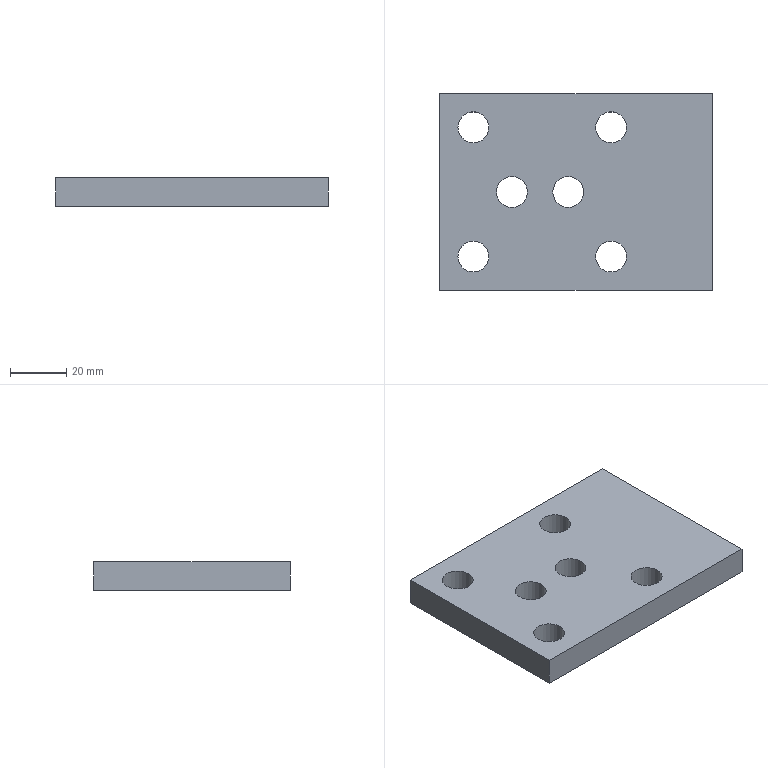Part | NX | features solid 2 | 1 solid | 12 faces | box 97 x 70 x 10 mm | volume 62198 mm3 | plane 6 | cylinder 6 | commonest cylinder face diameters 11 x6
STEP:
#1=CARTESIAN_POINT('',(1618.396,35.,88.));
#2=VERTEX_POINT('',#1);
#3=CARTESIAN_POINT('',(1618.396,35.,78.));
#4=VERTEX_POINT('',#3);
#5=CARTESIAN_POINT('',(1618.396,35.,78.));
#6=DIRECTION('',(0.,0.,1.));
#7=VECTOR('',#6,1000.);
#8=LINE('',#5,#7);
#9=EDGE_CURVE('',#2,#4,#8,.F.);
#10=ORIENTED_EDGE('',*,*,#9,.T.);
#11=CARTESIAN_POINT('',(1521.396,35.,78.));
#12=VERTEX_POINT('',#11);
#13=CARTESIAN_POINT('',(1569.896,35.,78.));
#14=DIRECTION('',(-1.,0.,0.));
#15=VECTOR('',#14,1000.);
#16=LINE('',#13,#15);
#17=EDGE_CURVE('',#12,#4,#16,.F.);
#18=ORIENTED_EDGE('',*,*,#17,.F.);
#19=CARTESIAN_POINT('',(1521.396,35.,88.));
#20=VERTEX_POINT('',#19);
#21=CARTESIAN_POINT('',(1521.396,35.,78.));
#22=DIRECTION('',(0.,0.,1.));
#23=VECTOR('',#22,1000.);
#24=LINE('',#21,#23);
#25=EDGE_CURVE('',#20,#12,#24,.F.);
#26=ORIENTED_EDGE('',*,*,#25,.F.);
#27=CARTESIAN_POINT('',(2186.158,35.,88.));
#28=DIRECTION('',(1.,0.,0.));
#29=VECTOR('',#28,1000.);
#30=LINE('',#27,#29);
#31=EDGE_CURVE('',#20,#2,#30,.T.);
#32=ORIENTED_EDGE('',*,*,#31,.T.);
#33=EDGE_LOOP('',(#10,#18,#26,#32));
#34=FACE_BOUND('',#33,.T.);
#35=CARTESIAN_POINT('',(1569.896,35.,78.));
#36=DIRECTION('',(0.,-1.,0.));
#37=DIRECTION('',(-1.,0.,0.));
#38=AXIS2_PLACEMENT_3D('',#35,#36,#37);
#39=PLANE('',#38);
#40=ADVANCED_FACE('',(#34),#39,.F.);
#41=ORIENTED_EDGE('',*,*,#25,.T.);
#42=CARTESIAN_POINT('',(1521.396,-35.,78.));
#43=VERTEX_POINT('',#42);
#44=CARTESIAN_POINT('',(1521.396,0.,78.));
#45=DIRECTION('',(0.,-1.,0.));
#46=VECTOR('',#45,1000.);
#47=LINE('',#44,#46);
#48=EDGE_CURVE('',#43,#12,#47,.F.);
#49=ORIENTED_EDGE('',*,*,#48,.F.);
#50=CARTESIAN_POINT('',(1521.396,-35.,88.));
#51=VERTEX_POINT('',#50);
#52=CARTESIAN_POINT('',(1521.396,-35.,78.));
#53=DIRECTION('',(0.,0.,1.));
#54=VECTOR('',#53,1000.);
#55=LINE('',#52,#54);
#56=EDGE_CURVE('',#51,#43,#55,.F.);
#57=ORIENTED_EDGE('',*,*,#56,.F.);
#58=CARTESIAN_POINT('',(1521.396,0.000000688,88.));
#59=DIRECTION('',(0.,-1.,0.));
#60=VECTOR('',#59,1000.);
#61=LINE('',#58,#60);
#62=EDGE_CURVE('',#51,#20,#61,.F.);
#63=ORIENTED_EDGE('',*,*,#62,.T.);
#64=EDGE_LOOP('',(#41,#49,#57,#63));
#65=FACE_BOUND('',#64,.T.);
#66=CARTESIAN_POINT('',(1521.396,0.,78.));
#67=DIRECTION('',(1.,0.,0.));
#68=DIRECTION('',(0.,-1.,0.));
#69=AXIS2_PLACEMENT_3D('',#66,#67,#68);
#70=PLANE('',#69);
#71=ADVANCED_FACE('',(#65),#70,.F.);
#72=ORIENTED_EDGE('',*,*,#56,.T.);
#73=CARTESIAN_POINT('',(1618.396,-35.,78.));
#74=VERTEX_POINT('',#73);
#75=CARTESIAN_POINT('',(1569.896,-35.,78.));
#76=DIRECTION('',(1.,0.,0.));
#77=VECTOR('',#76,1000.);
#78=LINE('',#75,#77);
#79=EDGE_CURVE('',#74,#43,#78,.F.);
#80=ORIENTED_EDGE('',*,*,#79,.F.);
#81=CARTESIAN_POINT('',(1618.396,-35.,88.));
#82=VERTEX_POINT('',#81);
#83=CARTESIAN_POINT('',(1618.396,-35.,78.));
#84=DIRECTION('',(0.,0.,1.));
#85=VECTOR('',#84,1000.);
#86=LINE('',#83,#85);
#87=EDGE_CURVE('',#82,#74,#86,.F.);
#88=ORIENTED_EDGE('',*,*,#87,.F.);
#89=CARTESIAN_POINT('',(2186.158,-35.,88.));
#90=DIRECTION('',(1.,0.,0.));
#91=VECTOR('',#90,1000.);
#92=LINE('',#89,#91);
#93=EDGE_CURVE('',#82,#51,#92,.F.);
#94=ORIENTED_EDGE('',*,*,#93,.T.);
#95=EDGE_LOOP('',(#72,#80,#88,#94));
#96=FACE_BOUND('',#95,.T.);
#97=CARTESIAN_POINT('',(1569.896,-35.,78.));
#98=DIRECTION('',(0.,1.,0.));
#99=DIRECTION('',(1.,0.,0.));
#100=AXIS2_PLACEMENT_3D('',#97,#98,#99);
#101=PLANE('',#100);
#102=ADVANCED_FACE('',(#96),#101,.F.);
#103=CARTESIAN_POINT('',(1527.896,23.,78.));
#104=VERTEX_POINT('',#103);
#105=CARTESIAN_POINT('',(1533.396,23.,78.));
#106=DIRECTION('',(0.,0.,-1.));
#107=DIRECTION('',(-1.,0.,0.));
#108=AXIS2_PLACEMENT_3D('',#105,#106,#107);
#109=CIRCLE('',#108,5.5);
#110=EDGE_CURVE('',#104,#104,#109,.T.);
#111=ORIENTED_EDGE('',*,*,#110,.T.);
#112=EDGE_LOOP('',(#111));
#113=FACE_BOUND('',#112,.T.);
#114=CARTESIAN_POINT('',(1527.896,23.,88.));
#115=VERTEX_POINT('',#114);
#116=CARTESIAN_POINT('',(1533.396,23.,88.));
#117=DIRECTION('',(0.,0.,-1.));
#118=DIRECTION('',(-1.,0.,0.));
#119=AXIS2_PLACEMENT_3D('',#116,#117,#118);
#120=CIRCLE('',#119,5.5);
#121=EDGE_CURVE('',#115,#115,#120,.T.);
#122=ORIENTED_EDGE('',*,*,#121,.F.);
#123=EDGE_LOOP('',(#122));
#124=FACE_BOUND('',#123,.T.);
#125=CARTESIAN_POINT('',(1533.396,23.,78.));
#126=DIRECTION('',(0.,0.,-1.));
#127=DIRECTION('',(-1.,0.,0.));
#128=AXIS2_PLACEMENT_3D('',#125,#126,#127);
#129=CYLINDRICAL_SURFACE('',#128,5.5);
#130=ADVANCED_FACE('',(#113,#124),#129,.F.);
#131=CARTESIAN_POINT('',(1576.896,23.,78.));
#132=VERTEX_POINT('',#131);
#133=CARTESIAN_POINT('',(1582.396,23.,78.));
#134=DIRECTION('',(0.,0.,-1.));
#135=DIRECTION('',(-1.,0.,0.));
#136=AXIS2_PLACEMENT_3D('',#133,#134,#135);
#137=CIRCLE('',#136,5.5);
#138=EDGE_CURVE('',#132,#132,#137,.T.);
#139=ORIENTED_EDGE('',*,*,#138,.T.);
#140=EDGE_LOOP('',(#139));
#141=FACE_BOUND('',#140,.T.);
#142=CARTESIAN_POINT('',(1576.896,23.,88.));
#143=VERTEX_POINT('',#142);
#144=CARTESIAN_POINT('',(1582.396,23.,88.));
#145=DIRECTION('',(0.,0.,-1.));
#146=DIRECTION('',(-1.,0.,0.));
#147=AXIS2_PLACEMENT_3D('',#144,#145,#146);
#148=CIRCLE('',#147,5.5);
#149=EDGE_CURVE('',#143,#143,#148,.T.);
#150=ORIENTED_EDGE('',*,*,#149,.F.);
#151=EDGE_LOOP('',(#150));
#152=FACE_BOUND('',#151,.T.);
#153=CARTESIAN_POINT('',(1582.396,23.,78.));
#154=DIRECTION('',(0.,0.,-1.));
#155=DIRECTION('',(-1.,0.,0.));
#156=AXIS2_PLACEMENT_3D('',#153,#154,#155);
#157=CYLINDRICAL_SURFACE('',#156,5.5);
#158=ADVANCED_FACE('',(#141,#152),#157,.F.);
#159=CARTESIAN_POINT('',(1576.896,-23.,78.));
#160=VERTEX_POINT('',#159);
#161=CARTESIAN_POINT('',(1582.396,-23.,78.));
#162=DIRECTION('',(0.,0.,-1.));
#163=DIRECTION('',(-1.,0.,0.));
#164=AXIS2_PLACEMENT_3D('',#161,#162,#163);
#165=CIRCLE('',#164,5.5);
#166=EDGE_CURVE('',#160,#160,#165,.T.);
#167=ORIENTED_EDGE('',*,*,#166,.T.);
#168=EDGE_LOOP('',(#167));
#169=FACE_BOUND('',#168,.T.);
#170=CARTESIAN_POINT('',(1576.896,-23.,88.));
#171=VERTEX_POINT('',#170);
#172=CARTESIAN_POINT('',(1582.396,-23.,88.));
#173=DIRECTION('',(0.,0.,-1.));
#174=DIRECTION('',(-1.,0.,0.));
#175=AXIS2_PLACEMENT_3D('',#172,#173,#174);
#176=CIRCLE('',#175,5.5);
#177=EDGE_CURVE('',#171,#171,#176,.T.);
#178=ORIENTED_EDGE('',*,*,#177,.F.);
#179=EDGE_LOOP('',(#178));
#180=FACE_BOUND('',#179,.T.);
#181=CARTESIAN_POINT('',(1582.396,-23.,78.));
#182=DIRECTION('',(0.,0.,-1.));
#183=DIRECTION('',(-1.,0.,0.));
#184=AXIS2_PLACEMENT_3D('',#181,#182,#183);
#185=CYLINDRICAL_SURFACE('',#184,5.5);
#186=ADVANCED_FACE('',(#169,#180),#185,.F.);
#187=CARTESIAN_POINT('',(1527.896,-23.,78.));
#188=VERTEX_POINT('',#187);
#189=CARTESIAN_POINT('',(1533.396,-23.,78.));
#190=DIRECTION('',(0.,0.,-1.));
#191=DIRECTION('',(-1.,0.,0.));
#192=AXIS2_PLACEMENT_3D('',#189,#190,#191);
#193=CIRCLE('',#192,5.5);
#194=EDGE_CURVE('',#188,#188,#193,.F.);
#195=ORIENTED_EDGE('',*,*,#194,.F.);
#196=EDGE_LOOP('',(#195));
#197=FACE_BOUND('',#196,.T.);
#198=CARTESIAN_POINT('',(1527.896,-23.,88.));
#199=VERTEX_POINT('',#198);
#200=CARTESIAN_POINT('',(1533.396,-23.,88.));
#201=DIRECTION('',(0.,0.,-1.));
#202=DIRECTION('',(-1.,0.,0.));
#203=AXIS2_PLACEMENT_3D('',#200,#201,#202);
#204=CIRCLE('',#203,5.5);
#205=EDGE_CURVE('',#199,#199,#204,.F.);
#206=ORIENTED_EDGE('',*,*,#205,.T.);
#207=EDGE_LOOP('',(#206));
#208=FACE_BOUND('',#207,.T.);
#209=CARTESIAN_POINT('',(1533.396,-23.,78.));
#210=DIRECTION('',(0.,0.,-1.));
#211=DIRECTION('',(-1.,0.,0.));
#212=AXIS2_PLACEMENT_3D('',#209,#210,#211);
#213=CYLINDRICAL_SURFACE('',#212,5.5);
#214=ADVANCED_FACE('',(#197,#208),#213,.F.);
#215=CARTESIAN_POINT('',(1618.396,0.000000688,88.));
#216=DIRECTION('',(0.,-1.,0.));
#217=VECTOR('',#216,1000.);
#218=LINE('',#215,#217);
#219=EDGE_CURVE('',#2,#82,#218,.T.);
#220=ORIENTED_EDGE('',*,*,#219,.T.);
#221=ORIENTED_EDGE('',*,*,#87,.T.);
#222=CARTESIAN_POINT('',(1618.396,0.,78.));
#223=DIRECTION('',(0.,1.,0.));
#224=VECTOR('',#223,1000.);
#225=LINE('',#222,#224);
#226=EDGE_CURVE('',#4,#74,#225,.F.);
#227=ORIENTED_EDGE('',*,*,#226,.F.);
#228=ORIENTED_EDGE('',*,*,#9,.F.);
#229=EDGE_LOOP('',(#220,#221,#227,#228));
#230=FACE_BOUND('',#229,.T.);
#231=CARTESIAN_POINT('',(1618.396,0.,78.));
#232=DIRECTION('',(-1.,0.,0.));
#233=DIRECTION('',(0.,1.,0.));
#234=AXIS2_PLACEMENT_3D('',#231,#232,#233);
#235=PLANE('',#234);
#236=ADVANCED_FACE('',(#230),#235,.F.);
#237=CARTESIAN_POINT('',(1572.616,0.,78.));
#238=VERTEX_POINT('',#237);
#239=CARTESIAN_POINT('',(1567.116,0.,78.));
#240=DIRECTION('',(0.,0.,1.));
#241=DIRECTION('',(1.,0.,0.));
#242=AXIS2_PLACEMENT_3D('',#239,#240,#241);
#243=CIRCLE('',#242,5.5);
#244=EDGE_CURVE('',#238,#238,#243,.T.);
#245=ORIENTED_EDGE('',*,*,#244,.T.);
#246=EDGE_LOOP('',(#245));
#247=FACE_BOUND('',#246,.T.);
#248=CARTESIAN_POINT('',(1552.616,0.,78.));
#249=VERTEX_POINT('',#248);
#250=CARTESIAN_POINT('',(1547.116,0.,78.));
#251=DIRECTION('',(0.,0.,1.));
#252=DIRECTION('',(1.,0.,0.));
#253=AXIS2_PLACEMENT_3D('',#250,#251,#252);
#254=CIRCLE('',#253,5.5);
#255=EDGE_CURVE('',#249,#249,#254,.T.);
#256=ORIENTED_EDGE('',*,*,#255,.T.);
#257=EDGE_LOOP('',(#256));
#258=FACE_BOUND('',#257,.T.);
#259=ORIENTED_EDGE('',*,*,#110,.F.);
#260=EDGE_LOOP('',(#259));
#261=FACE_BOUND('',#260,.T.);
#262=ORIENTED_EDGE('',*,*,#138,.F.);
#263=EDGE_LOOP('',(#262));
#264=FACE_BOUND('',#263,.T.);
#265=ORIENTED_EDGE('',*,*,#166,.F.);
#266=EDGE_LOOP('',(#265));
#267=FACE_BOUND('',#266,.T.);
#268=ORIENTED_EDGE('',*,*,#194,.T.);
#269=EDGE_LOOP('',(#268));
#270=FACE_BOUND('',#269,.T.);
#271=ORIENTED_EDGE('',*,*,#79,.T.);
#272=ORIENTED_EDGE('',*,*,#48,.T.);
#273=ORIENTED_EDGE('',*,*,#17,.T.);
#274=ORIENTED_EDGE('',*,*,#226,.T.);
#275=EDGE_LOOP('',(#271,#272,#273,#274));
#276=FACE_BOUND('',#275,.T.);
#277=CARTESIAN_POINT('',(2186.158,0.000000688,78.));
#278=DIRECTION('',(0.,0.,-1.));
#279=DIRECTION('',(1.,0.,0.));
#280=AXIS2_PLACEMENT_3D('',#277,#278,#279);
#281=PLANE('',#280);
#282=ADVANCED_FACE('',(#247,#258,#261,#264,#267,#270,#276),#281,.T.);
#283=CARTESIAN_POINT('',(1561.616,0.,88.));
#284=VERTEX_POINT('',#283);
#285=CARTESIAN_POINT('',(1567.116,0.,88.));
#286=DIRECTION('',(0.,0.,-1.));
#287=DIRECTION('',(-1.,0.,0.));
#288=AXIS2_PLACEMENT_3D('',#285,#286,#287);
#289=CIRCLE('',#288,5.5);
#290=EDGE_CURVE('',#284,#284,#289,.F.);
#291=ORIENTED_EDGE('',*,*,#290,.F.);
#292=EDGE_LOOP('',(#291));
#293=FACE_BOUND('',#292,.T.);
#294=CARTESIAN_POINT('',(1541.616,0.,88.));
#295=VERTEX_POINT('',#294);
#296=CARTESIAN_POINT('',(1547.116,0.,88.));
#297=DIRECTION('',(0.,0.,-1.));
#298=DIRECTION('',(-1.,0.,0.));
#299=AXIS2_PLACEMENT_3D('',#296,#297,#298);
#300=CIRCLE('',#299,5.5);
#301=EDGE_CURVE('',#295,#295,#300,.F.);
#302=ORIENTED_EDGE('',*,*,#301,.F.);
#303=EDGE_LOOP('',(#302));
#304=FACE_BOUND('',#303,.T.);
#305=ORIENTED_EDGE('',*,*,#121,.T.);
#306=EDGE_LOOP('',(#305));
#307=FACE_BOUND('',#306,.T.);
#308=ORIENTED_EDGE('',*,*,#149,.T.);
#309=EDGE_LOOP('',(#308));
#310=FACE_BOUND('',#309,.T.);
#311=ORIENTED_EDGE('',*,*,#177,.T.);
#312=EDGE_LOOP('',(#311));
#313=FACE_BOUND('',#312,.T.);
#314=ORIENTED_EDGE('',*,*,#205,.F.);
#315=EDGE_LOOP('',(#314));
#316=FACE_BOUND('',#315,.T.);
#317=ORIENTED_EDGE('',*,*,#93,.F.);
#318=ORIENTED_EDGE('',*,*,#219,.F.);
#319=ORIENTED_EDGE('',*,*,#31,.F.);
#320=ORIENTED_EDGE('',*,*,#62,.F.);
#321=EDGE_LOOP('',(#317,#318,#319,#320));
#322=FACE_BOUND('',#321,.T.);
#323=CARTESIAN_POINT('',(2186.158,0.000000688,88.));
#324=DIRECTION('',(0.,0.,-1.));
#325=DIRECTION('',(1.,0.,0.));
#326=AXIS2_PLACEMENT_3D('',#323,#324,#325);
#327=PLANE('',#326);
#328=ADVANCED_FACE('',(#293,#304,#307,#310,#313,#316,#322),#327,.F.);
#329=ORIENTED_EDGE('',*,*,#301,.T.);
#330=EDGE_LOOP('',(#329));
#331=FACE_BOUND('',#330,.T.);
#332=ORIENTED_EDGE('',*,*,#255,.F.);
#333=EDGE_LOOP('',(#332));
#334=FACE_BOUND('',#333,.T.);
#335=CARTESIAN_POINT('',(1547.116,0.,78.));
#336=DIRECTION('',(0.,0.,1.));
#337=DIRECTION('',(1.,0.,0.));
#338=AXIS2_PLACEMENT_3D('',#335,#336,#337);
#339=CYLINDRICAL_SURFACE('',#338,5.5);
#340=ADVANCED_FACE('',(#331,#334),#339,.F.);
#341=ORIENTED_EDGE('',*,*,#290,.T.);
#342=EDGE_LOOP('',(#341));
#343=FACE_BOUND('',#342,.T.);
#344=ORIENTED_EDGE('',*,*,#244,.F.);
#345=EDGE_LOOP('',(#344));
#346=FACE_BOUND('',#345,.T.);
#347=CARTESIAN_POINT('',(1567.116,0.,78.));
#348=DIRECTION('',(0.,0.,1.));
#349=DIRECTION('',(1.,0.,0.));
#350=AXIS2_PLACEMENT_3D('',#347,#348,#349);
#351=CYLINDRICAL_SURFACE('',#350,5.5);
#352=ADVANCED_FACE('',(#343,#346),#351,.F.);
#353=CLOSED_SHELL('',(#40,#71,#102,#130,#158,#186,#214,#236,#282,#328,#340,#352));
#354=MANIFOLD_SOLID_BREP('',#353);
#355=(LENGTH_UNIT()NAMED_UNIT(*)SI_UNIT(.MILLI.,.METRE.));
#356=UNCERTAINTY_MEASURE_WITH_UNIT(LENGTH_MEASURE(0.00001),#355,'','');
#357=(NAMED_UNIT(*)PLANE_ANGLE_UNIT()SI_UNIT($,.RADIAN.));
#358=(NAMED_UNIT(*)SI_UNIT($,.STERADIAN.)SOLID_ANGLE_UNIT());
#359=(GEOMETRIC_REPRESENTATION_CONTEXT(3)GLOBAL_UNCERTAINTY_ASSIGNED_CONTEXT((#356))GLOBAL_UNIT_ASSIGNED_CONTEXT((#355,#357,#358))REPRESENTATION_CONTEXT('',''));
#360=ADVANCED_BREP_SHAPE_REPRESENTATION('',(#354),#359);